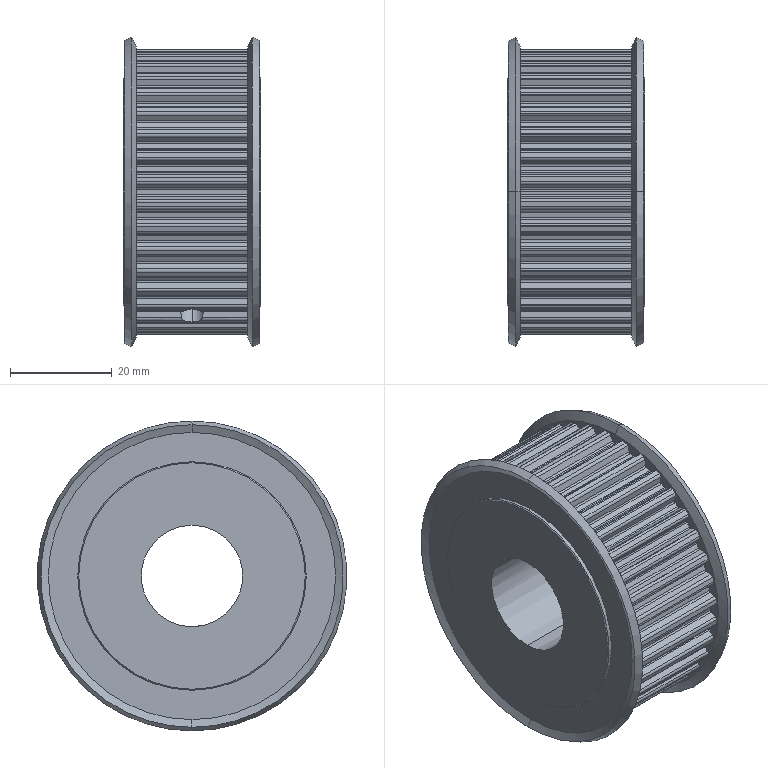Part | SolidWorks | 3 solids | 406 faces | box 27 x 61 x 61 mm | volume 54913 mm3 | cylinder 270 | plane 110 | cone 26 | commonest cylinder face diameters 0.8 x91 1.2 x90 52.85 x39 56.45 x36 4.917 x4 6 x4